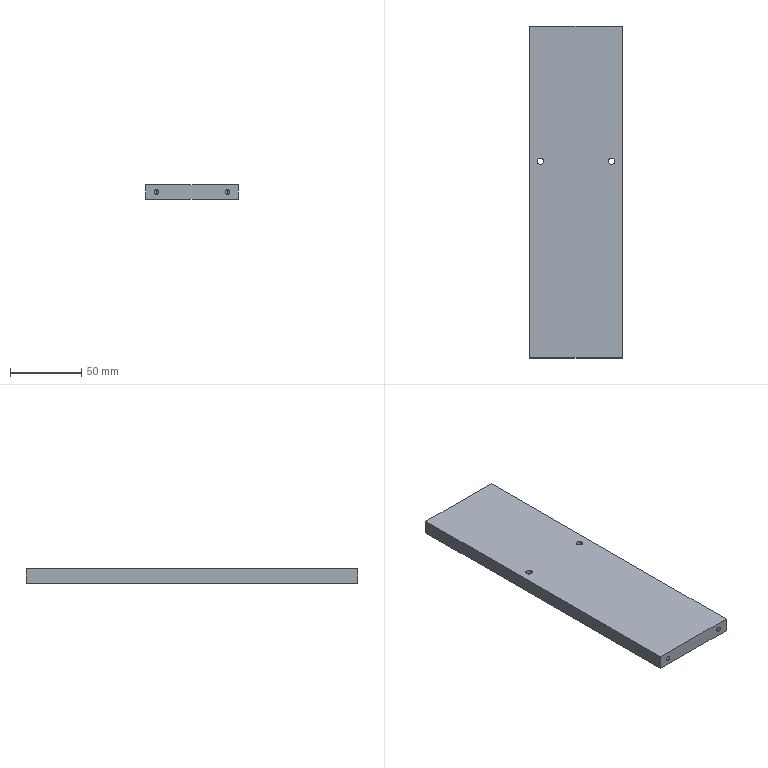Part | SolidWorks | features HoleWzd 2, Extrusion 1, MirrorPattern 1 | 1 solid | 26 faces | box 65 x 233 x 10 mm | volume 150775 mm3 | cylinder 12 | cone 8 | plane 6 | commonest cylinder face diameters 3.3 x8 4.5 x4
STEP:
#1=CARTESIAN_POINT('',(-22.75,21.5,5.));
#2=VERTEX_POINT('',#1);
#3=CARTESIAN_POINT('',(-27.25,21.5,5.));
#4=VERTEX_POINT('',#3);
#5=CARTESIAN_POINT('',(-25.,21.5,5.));
#6=DIRECTION('',(0.,0.,-1.));
#7=DIRECTION('',(-1.,0.,0.));
#8=AXIS2_PLACEMENT_3D('',#5,#6,#7);
#9=CIRCLE('',#8,2.25);
#10=EDGE_CURVE('',#2,#4,#9,.T.);
#11=ORIENTED_EDGE('',*,*,#10,.F.);
#12=CARTESIAN_POINT('',(-22.75,21.5,-5.));
#13=VERTEX_POINT('',#12);
#14=CARTESIAN_POINT('',(-22.75,21.5,-5.));
#15=DIRECTION('',(0.,0.,-1.));
#16=VECTOR('',#15,1000.);
#17=LINE('',#14,#16);
#18=EDGE_CURVE('',#2,#13,#17,.T.);
#19=ORIENTED_EDGE('',*,*,#18,.T.);
#20=CARTESIAN_POINT('',(-27.25,21.5,-5.));
#21=VERTEX_POINT('',#20);
#22=CARTESIAN_POINT('',(-25.,21.5,-5.));
#23=DIRECTION('',(0.,0.,-1.));
#24=DIRECTION('',(-1.,0.,0.));
#25=AXIS2_PLACEMENT_3D('',#22,#23,#24);
#26=CIRCLE('',#25,2.25);
#27=EDGE_CURVE('',#13,#21,#26,.T.);
#28=ORIENTED_EDGE('',*,*,#27,.T.);
#29=CARTESIAN_POINT('',(-27.25,21.5,-5.));
#30=DIRECTION('',(0.,0.,-1.));
#31=VECTOR('',#30,1000.);
#32=LINE('',#29,#31);
#33=EDGE_CURVE('',#4,#21,#32,.T.);
#34=ORIENTED_EDGE('',*,*,#33,.F.);
#35=EDGE_LOOP('',(#11,#19,#28,#34));
#36=FACE_OUTER_BOUND('',#35,.T.);
#37=CARTESIAN_POINT('',(-25.,21.5,-5.));
#38=DIRECTION('',(0.,0.,-1.));
#39=DIRECTION('',(-1.,0.,0.));
#40=AXIS2_PLACEMENT_3D('',#37,#38,#39);
#41=CYLINDRICAL_SURFACE('',#40,2.25);
#42=ADVANCED_FACE('',(#36),#41,.F.);
#43=CARTESIAN_POINT('',(27.25,21.5,5.));
#44=VERTEX_POINT('',#43);
#45=CARTESIAN_POINT('',(22.75,21.5,5.));
#46=VERTEX_POINT('',#45);
#47=CARTESIAN_POINT('',(25.,21.5,5.));
#48=DIRECTION('',(0.,0.,-1.));
#49=DIRECTION('',(-1.,0.,0.));
#50=AXIS2_PLACEMENT_3D('',#47,#48,#49);
#51=CIRCLE('',#50,2.25);
#52=EDGE_CURVE('',#44,#46,#51,.T.);
#53=ORIENTED_EDGE('',*,*,#52,.F.);
#54=CARTESIAN_POINT('',(27.25,21.5,-5.));
#55=VERTEX_POINT('',#54);
#56=CARTESIAN_POINT('',(27.25,21.5,-5.));
#57=DIRECTION('',(0.,0.,-1.));
#58=VECTOR('',#57,1000.);
#59=LINE('',#56,#58);
#60=EDGE_CURVE('',#44,#55,#59,.T.);
#61=ORIENTED_EDGE('',*,*,#60,.T.);
#62=CARTESIAN_POINT('',(22.75,21.5,-5.));
#63=VERTEX_POINT('',#62);
#64=CARTESIAN_POINT('',(25.,21.5,-5.));
#65=DIRECTION('',(0.,0.,-1.));
#66=DIRECTION('',(-1.,0.,0.));
#67=AXIS2_PLACEMENT_3D('',#64,#65,#66);
#68=CIRCLE('',#67,2.25);
#69=EDGE_CURVE('',#55,#63,#68,.T.);
#70=ORIENTED_EDGE('',*,*,#69,.T.);
#71=CARTESIAN_POINT('',(22.75,21.5,-5.));
#72=DIRECTION('',(0.,0.,-1.));
#73=VECTOR('',#72,1000.);
#74=LINE('',#71,#73);
#75=EDGE_CURVE('',#46,#63,#74,.T.);
#76=ORIENTED_EDGE('',*,*,#75,.F.);
#77=EDGE_LOOP('',(#53,#61,#70,#76));
#78=FACE_OUTER_BOUND('',#77,.T.);
#79=CARTESIAN_POINT('',(25.,21.5,-5.));
#80=DIRECTION('',(0.,0.,-1.));
#81=DIRECTION('',(-1.,0.,0.));
#82=AXIS2_PLACEMENT_3D('',#79,#80,#81);
#83=CYLINDRICAL_SURFACE('',#82,2.25);
#84=ADVANCED_FACE('',(#78),#83,.F.);
#85=CARTESIAN_POINT('',(25.,-106.4,1.65));
#86=VERTEX_POINT('',#85);
#87=CARTESIAN_POINT('',(25.,-106.4,-1.65));
#88=VERTEX_POINT('',#87);
#89=CARTESIAN_POINT('',(25.,-106.4,0.));
#90=DIRECTION('',(0.,-1.,0.));
#91=DIRECTION('',(0.,0.,-1.));
#92=AXIS2_PLACEMENT_3D('',#89,#90,#91);
#93=CIRCLE('',#92,1.65);
#94=EDGE_CURVE('',#86,#88,#93,.T.);
#95=ORIENTED_EDGE('',*,*,#94,.F.);
#96=CARTESIAN_POINT('',(25.,-116.5,1.65));
#97=VERTEX_POINT('',#96);
#98=CARTESIAN_POINT('',(25.,-116.5,1.65));
#99=DIRECTION('',(0.,-1.,0.));
#100=VECTOR('',#99,1000.);
#101=LINE('',#98,#100);
#102=EDGE_CURVE('',#86,#97,#101,.T.);
#103=ORIENTED_EDGE('',*,*,#102,.T.);
#104=CARTESIAN_POINT('',(25.,-116.5,-1.65));
#105=VERTEX_POINT('',#104);
#106=CARTESIAN_POINT('',(25.,-116.5,0.));
#107=DIRECTION('',(0.,-1.,0.));
#108=DIRECTION('',(0.,0.,-1.));
#109=AXIS2_PLACEMENT_3D('',#106,#107,#108);
#110=CIRCLE('',#109,1.65);
#111=EDGE_CURVE('',#97,#105,#110,.T.);
#112=ORIENTED_EDGE('',*,*,#111,.T.);
#113=CARTESIAN_POINT('',(25.,-116.5,-1.65));
#114=DIRECTION('',(0.,-1.,0.));
#115=VECTOR('',#114,1000.);
#116=LINE('',#113,#115);
#117=EDGE_CURVE('',#88,#105,#116,.T.);
#118=ORIENTED_EDGE('',*,*,#117,.F.);
#119=EDGE_LOOP('',(#95,#103,#112,#118));
#120=FACE_OUTER_BOUND('',#119,.T.);
#121=CARTESIAN_POINT('',(25.,-116.5,0.));
#122=DIRECTION('',(0.,-1.,0.));
#123=DIRECTION('',(0.,0.,-1.));
#124=AXIS2_PLACEMENT_3D('',#121,#122,#123);
#125=CYLINDRICAL_SURFACE('',#124,1.65);
#126=ADVANCED_FACE('',(#120),#125,.F.);
#127=CARTESIAN_POINT('',(25.,-105.409,0.));
#128=VERTEX_POINT('',#127);
#129=CARTESIAN_POINT('',(25.,-106.4,-1.65));
#130=DIRECTION('',(0.,-0.515,-0.8572));
#131=VECTOR('',#130,1000.);
#132=LINE('',#129,#131);
#133=EDGE_CURVE('',#128,#88,#132,.T.);
#134=ORIENTED_EDGE('',*,*,#133,.F.);
#135=CARTESIAN_POINT('',(25.,-106.4,1.65));
#136=DIRECTION('',(0.,-0.515,0.8572));
#137=VECTOR('',#136,1000.);
#138=LINE('',#135,#137);
#139=EDGE_CURVE('',#128,#86,#138,.T.);
#140=ORIENTED_EDGE('',*,*,#139,.T.);
#141=ORIENTED_EDGE('',*,*,#94,.T.);
#142=EDGE_LOOP('',(#134,#140,#141));
#143=FACE_OUTER_BOUND('',#142,.T.);
#144=CARTESIAN_POINT('',(25.,-106.4,0.));
#145=DIRECTION('',(0.,-1.,0.));
#146=DIRECTION('',(0.,0.,-1.));
#147=AXIS2_PLACEMENT_3D('',#144,#145,#146);
#148=CONICAL_SURFACE('',#147,1.65,1.03);
#149=ADVANCED_FACE('',(#143),#148,.F.);
#150=CARTESIAN_POINT('',(-25.,-106.4,1.65));
#151=VERTEX_POINT('',#150);
#152=CARTESIAN_POINT('',(-25.,-106.4,-1.65));
#153=VERTEX_POINT('',#152);
#154=CARTESIAN_POINT('',(-25.,-106.4,0.));
#155=DIRECTION('',(0.,-1.,0.));
#156=DIRECTION('',(0.,0.,-1.));
#157=AXIS2_PLACEMENT_3D('',#154,#155,#156);
#158=CIRCLE('',#157,1.65);
#159=EDGE_CURVE('',#151,#153,#158,.T.);
#160=ORIENTED_EDGE('',*,*,#159,.F.);
#161=CARTESIAN_POINT('',(-25.,-116.5,1.65));
#162=VERTEX_POINT('',#161);
#163=CARTESIAN_POINT('',(-25.,-116.5,1.65));
#164=DIRECTION('',(0.,-1.,0.));
#165=VECTOR('',#164,1000.);
#166=LINE('',#163,#165);
#167=EDGE_CURVE('',#151,#162,#166,.T.);
#168=ORIENTED_EDGE('',*,*,#167,.T.);
#169=CARTESIAN_POINT('',(-25.,-116.5,-1.65));
#170=VERTEX_POINT('',#169);
#171=CARTESIAN_POINT('',(-25.,-116.5,0.));
#172=DIRECTION('',(0.,-1.,0.));
#173=DIRECTION('',(0.,0.,-1.));
#174=AXIS2_PLACEMENT_3D('',#171,#172,#173);
#175=CIRCLE('',#174,1.65);
#176=EDGE_CURVE('',#162,#170,#175,.T.);
#177=ORIENTED_EDGE('',*,*,#176,.T.);
#178=CARTESIAN_POINT('',(-25.,-116.5,-1.65));
#179=DIRECTION('',(0.,-1.,0.));
#180=VECTOR('',#179,1000.);
#181=LINE('',#178,#180);
#182=EDGE_CURVE('',#153,#170,#181,.T.);
#183=ORIENTED_EDGE('',*,*,#182,.F.);
#184=EDGE_LOOP('',(#160,#168,#177,#183));
#185=FACE_OUTER_BOUND('',#184,.T.);
#186=CARTESIAN_POINT('',(-25.,-116.5,0.));
#187=DIRECTION('',(0.,-1.,0.));
#188=DIRECTION('',(0.,0.,-1.));
#189=AXIS2_PLACEMENT_3D('',#186,#187,#188);
#190=CYLINDRICAL_SURFACE('',#189,1.65);
#191=ADVANCED_FACE('',(#185),#190,.F.);
#192=CARTESIAN_POINT('',(-25.,-105.409,0.));
#193=VERTEX_POINT('',#192);
#194=CARTESIAN_POINT('',(-25.,-106.4,-1.65));
#195=DIRECTION('',(0.,-0.515,-0.8572));
#196=VECTOR('',#195,1000.);
#197=LINE('',#194,#196);
#198=EDGE_CURVE('',#193,#153,#197,.T.);
#199=ORIENTED_EDGE('',*,*,#198,.F.);
#200=CARTESIAN_POINT('',(-25.,-106.4,1.65));
#201=DIRECTION('',(0.,-0.515,0.8572));
#202=VECTOR('',#201,1000.);
#203=LINE('',#200,#202);
#204=EDGE_CURVE('',#193,#151,#203,.T.);
#205=ORIENTED_EDGE('',*,*,#204,.T.);
#206=ORIENTED_EDGE('',*,*,#159,.T.);
#207=EDGE_LOOP('',(#199,#205,#206));
#208=FACE_OUTER_BOUND('',#207,.T.);
#209=CARTESIAN_POINT('',(-25.,-106.4,0.));
#210=DIRECTION('',(0.,-1.,0.));
#211=DIRECTION('',(0.,0.,-1.));
#212=AXIS2_PLACEMENT_3D('',#209,#210,#211);
#213=CONICAL_SURFACE('',#212,1.65,1.03);
#214=ADVANCED_FACE('',(#208),#213,.F.);
#215=CARTESIAN_POINT('',(25.,106.4,-1.65));
#216=VERTEX_POINT('',#215);
#217=CARTESIAN_POINT('',(25.,106.4,1.65));
#218=VERTEX_POINT('',#217);
#219=CARTESIAN_POINT('',(25.,106.4,0.));
#220=DIRECTION('',(0.,1.,0.));
#221=DIRECTION('',(0.,0.,1.));
#222=AXIS2_PLACEMENT_3D('',#219,#220,#221);
#223=CIRCLE('',#222,1.65);
#224=EDGE_CURVE('',#216,#218,#223,.T.);
#225=ORIENTED_EDGE('',*,*,#224,.F.);
#226=CARTESIAN_POINT('',(25.,116.5,-1.65));
#227=VERTEX_POINT('',#226);
#228=CARTESIAN_POINT('',(25.,116.5,-1.65));
#229=DIRECTION('',(0.,1.,0.));
#230=VECTOR('',#229,1000.);
#231=LINE('',#228,#230);
#232=EDGE_CURVE('',#216,#227,#231,.T.);
#233=ORIENTED_EDGE('',*,*,#232,.T.);
#234=CARTESIAN_POINT('',(25.,116.5,1.65));
#235=VERTEX_POINT('',#234);
#236=CARTESIAN_POINT('',(25.,116.5,0.));
#237=DIRECTION('',(0.,1.,0.));
#238=DIRECTION('',(0.,0.,1.));
#239=AXIS2_PLACEMENT_3D('',#236,#237,#238);
#240=CIRCLE('',#239,1.65);
#241=EDGE_CURVE('',#227,#235,#240,.T.);
#242=ORIENTED_EDGE('',*,*,#241,.T.);
#243=CARTESIAN_POINT('',(25.,116.5,1.65));
#244=DIRECTION('',(0.,1.,0.));
#245=VECTOR('',#244,1000.);
#246=LINE('',#243,#245);
#247=EDGE_CURVE('',#218,#235,#246,.T.);
#248=ORIENTED_EDGE('',*,*,#247,.F.);
#249=EDGE_LOOP('',(#225,#233,#242,#248));
#250=FACE_OUTER_BOUND('',#249,.T.);
#251=CARTESIAN_POINT('',(25.,116.5,0.));
#252=DIRECTION('',(0.,1.,0.));
#253=DIRECTION('',(0.,0.,1.));
#254=AXIS2_PLACEMENT_3D('',#251,#252,#253);
#255=CYLINDRICAL_SURFACE('',#254,1.65);
#256=ADVANCED_FACE('',(#250),#255,.F.);
#257=CARTESIAN_POINT('',(25.,105.409,0.));
#258=VERTEX_POINT('',#257);
#259=CARTESIAN_POINT('',(25.,106.4,1.65));
#260=DIRECTION('',(0.,0.515,0.8572));
#261=VECTOR('',#260,1000.);
#262=LINE('',#259,#261);
#263=EDGE_CURVE('',#258,#218,#262,.T.);
#264=ORIENTED_EDGE('',*,*,#263,.F.);
#265=CARTESIAN_POINT('',(25.,106.4,-1.65));
#266=DIRECTION('',(0.,0.515,-0.8572));
#267=VECTOR('',#266,1000.);
#268=LINE('',#265,#267);
#269=EDGE_CURVE('',#258,#216,#268,.T.);
#270=ORIENTED_EDGE('',*,*,#269,.T.);
#271=ORIENTED_EDGE('',*,*,#224,.T.);
#272=EDGE_LOOP('',(#264,#270,#271));
#273=FACE_OUTER_BOUND('',#272,.T.);
#274=CARTESIAN_POINT('',(25.,106.4,0.));
#275=DIRECTION('',(0.,1.,0.));
#276=DIRECTION('',(0.,0.,1.));
#277=AXIS2_PLACEMENT_3D('',#274,#275,#276);
#278=CONICAL_SURFACE('',#277,1.65,1.03);
#279=ADVANCED_FACE('',(#273),#278,.F.);
#280=CARTESIAN_POINT('',(-25.,106.4,-1.65));
#281=VERTEX_POINT('',#280);
#282=CARTESIAN_POINT('',(-25.,106.4,1.65));
#283=VERTEX_POINT('',#282);
#284=CARTESIAN_POINT('',(-25.,106.4,0.));
#285=DIRECTION('',(0.,1.,0.));
#286=DIRECTION('',(0.,0.,1.));
#287=AXIS2_PLACEMENT_3D('',#284,#285,#286);
#288=CIRCLE('',#287,1.65);
#289=EDGE_CURVE('',#281,#283,#288,.T.);
#290=ORIENTED_EDGE('',*,*,#289,.F.);
#291=CARTESIAN_POINT('',(-25.,116.5,-1.65));
#292=VERTEX_POINT('',#291);
#293=CARTESIAN_POINT('',(-25.,116.5,-1.65));
#294=DIRECTION('',(0.,1.,0.));
#295=VECTOR('',#294,1000.);
#296=LINE('',#293,#295);
#297=EDGE_CURVE('',#281,#292,#296,.T.);
#298=ORIENTED_EDGE('',*,*,#297,.T.);
#299=CARTESIAN_POINT('',(-25.,116.5,1.65));
#300=VERTEX_POINT('',#299);
#301=CARTESIAN_POINT('',(-25.,116.5,0.));
#302=DIRECTION('',(0.,1.,0.));
#303=DIRECTION('',(0.,0.,1.));
#304=AXIS2_PLACEMENT_3D('',#301,#302,#303);
#305=CIRCLE('',#304,1.65);
#306=EDGE_CURVE('',#292,#300,#305,.T.);
#307=ORIENTED_EDGE('',*,*,#306,.T.);
#308=CARTESIAN_POINT('',(-25.,116.5,1.65));
#309=DIRECTION('',(0.,1.,0.));
#310=VECTOR('',#309,1000.);
#311=LINE('',#308,#310);
#312=EDGE_CURVE('',#283,#300,#311,.T.);
#313=ORIENTED_EDGE('',*,*,#312,.F.);
#314=EDGE_LOOP('',(#290,#298,#307,#313));
#315=FACE_OUTER_BOUND('',#314,.T.);
#316=CARTESIAN_POINT('',(-25.,116.5,0.));
#317=DIRECTION('',(0.,1.,0.));
#318=DIRECTION('',(0.,0.,1.));
#319=AXIS2_PLACEMENT_3D('',#316,#317,#318);
#320=CYLINDRICAL_SURFACE('',#319,1.65);
#321=ADVANCED_FACE('',(#315),#320,.F.);
#322=CARTESIAN_POINT('',(-25.,105.409,0.));
#323=VERTEX_POINT('',#322);
#324=CARTESIAN_POINT('',(-25.,106.4,1.65));
#325=DIRECTION('',(0.,0.515,0.8572));
#326=VECTOR('',#325,1000.);
#327=LINE('',#324,#326);
#328=EDGE_CURVE('',#323,#283,#327,.T.);
#329=ORIENTED_EDGE('',*,*,#328,.F.);
#330=CARTESIAN_POINT('',(-25.,106.4,-1.65));
#331=DIRECTION('',(0.,0.515,-0.8572));
#332=VECTOR('',#331,1000.);
#333=LINE('',#330,#332);
#334=EDGE_CURVE('',#323,#281,#333,.T.);
#335=ORIENTED_EDGE('',*,*,#334,.T.);
#336=ORIENTED_EDGE('',*,*,#289,.T.);
#337=EDGE_LOOP('',(#329,#335,#336));
#338=FACE_OUTER_BOUND('',#337,.T.);
#339=CARTESIAN_POINT('',(-25.,106.4,0.));
#340=DIRECTION('',(0.,1.,0.));
#341=DIRECTION('',(0.,0.,1.));
#342=AXIS2_PLACEMENT_3D('',#339,#340,#341);
#343=CONICAL_SURFACE('',#342,1.65,1.03);
#344=ADVANCED_FACE('',(#338),#343,.F.);
#345=CARTESIAN_POINT('',(32.5,-116.5,5.));
#346=VERTEX_POINT('',#345);
#347=CARTESIAN_POINT('',(32.5,-116.5,-5.));
#348=VERTEX_POINT('',#347);
#349=CARTESIAN_POINT('',(32.5,-116.5,-5.));
#350=DIRECTION('',(0.,0.,-1.));
#351=VECTOR('',#350,1000.);
#352=LINE('',#349,#351);
#353=EDGE_CURVE('',#346,#348,#352,.T.);
#354=ORIENTED_EDGE('',*,*,#353,.T.);
#355=CARTESIAN_POINT('',(32.5,116.5,-5.));
#356=VERTEX_POINT('',#355);
#357=CARTESIAN_POINT('',(32.5,116.5,-5.));
#358=DIRECTION('',(0.,-1.,0.));
#359=VECTOR('',#358,1000.);
#360=LINE('',#357,#359);
#361=EDGE_CURVE('',#356,#348,#360,.T.);
#362=ORIENTED_EDGE('',*,*,#361,.F.);
#363=CARTESIAN_POINT('',(32.5,116.5,5.));
#364=VERTEX_POINT('',#363);
#365=CARTESIAN_POINT('',(32.5,116.5,-5.));
#366=DIRECTION('',(0.,0.,-1.));
#367=VECTOR('',#366,1000.);
#368=LINE('',#365,#367);
#369=EDGE_CURVE('',#364,#356,#368,.T.);
#370=ORIENTED_EDGE('',*,*,#369,.F.);
#371=CARTESIAN_POINT('',(32.5,116.5,5.));
#372=DIRECTION('',(0.,-1.,0.));
#373=VECTOR('',#372,1000.);
#374=LINE('',#371,#373);
#375=EDGE_CURVE('',#364,#346,#374,.T.);
#376=ORIENTED_EDGE('',*,*,#375,.T.);
#377=EDGE_LOOP('',(#354,#362,#370,#376));
#378=FACE_OUTER_BOUND('',#377,.T.);
#379=CARTESIAN_POINT('',(32.5,116.5,-5.));
#380=DIRECTION('',(-1.,0.,0.));
#381=DIRECTION('',(0.,0.,1.));
#382=AXIS2_PLACEMENT_3D('',#379,#380,#381);
#383=PLANE('',#382);
#384=ADVANCED_FACE('',(#378),#383,.F.);
#385=CARTESIAN_POINT('',(-25.,21.5,-5.));
#386=DIRECTION('',(0.,0.,-1.));
#387=DIRECTION('',(-1.,0.,0.));
#388=AXIS2_PLACEMENT_3D('',#385,#386,#387);
#389=CIRCLE('',#388,2.25);
#390=EDGE_CURVE('',#21,#13,#389,.T.);
#391=ORIENTED_EDGE('',*,*,#390,.F.);
#392=ORIENTED_EDGE('',*,*,#27,.F.);
#393=EDGE_LOOP('',(#391,#392));
#394=FACE_BOUND('',#393,.T.);
#395=CARTESIAN_POINT('',(25.,21.5,-5.));
#396=DIRECTION('',(0.,0.,-1.));
#397=DIRECTION('',(-1.,0.,0.));
#398=AXIS2_PLACEMENT_3D('',#395,#396,#397);
#399=CIRCLE('',#398,2.25);
#400=EDGE_CURVE('',#63,#55,#399,.T.);
#401=ORIENTED_EDGE('',*,*,#400,.F.);
#402=ORIENTED_EDGE('',*,*,#69,.F.);
#403=EDGE_LOOP('',(#401,#402));
#404=FACE_BOUND('',#403,.T.);
#405=CARTESIAN_POINT('',(-32.5,-116.5,-5.));
#406=VERTEX_POINT('',#405);
#407=CARTESIAN_POINT('',(-32.5,-116.5,-5.));
#408=DIRECTION('',(-1.,0.,0.));
#409=VECTOR('',#408,1000.);
#410=LINE('',#407,#409);
#411=EDGE_CURVE('',#348,#406,#410,.T.);
#412=ORIENTED_EDGE('',*,*,#411,.T.);
#413=CARTESIAN_POINT('',(-32.5,116.5,-5.));
#414=VERTEX_POINT('',#413);
#415=CARTESIAN_POINT('',(-32.5,116.5,-5.));
#416=DIRECTION('',(0.,-1.,0.));
#417=VECTOR('',#416,1000.);
#418=LINE('',#415,#417);
#419=EDGE_CURVE('',#414,#406,#418,.T.);
#420=ORIENTED_EDGE('',*,*,#419,.F.);
#421=CARTESIAN_POINT('',(-32.5,116.5,-5.));
#422=DIRECTION('',(-1.,0.,0.));
#423=VECTOR('',#422,1000.);
#424=LINE('',#421,#423);
#425=EDGE_CURVE('',#356,#414,#424,.T.);
#426=ORIENTED_EDGE('',*,*,#425,.F.);
#427=ORIENTED_EDGE('',*,*,#361,.T.);
#428=EDGE_LOOP('',(#412,#420,#426,#427));
#429=FACE_OUTER_BOUND('',#428,.T.);
#430=CARTESIAN_POINT('',(-32.5,116.5,-5.));
#431=DIRECTION('',(0.,0.,1.));
#432=DIRECTION('',(1.,0.,0.));
#433=AXIS2_PLACEMENT_3D('',#430,#431,#432);
#434=PLANE('',#433);
#435=ADVANCED_FACE('',(#394,#404,#429),#434,.F.);
#436=CARTESIAN_POINT('',(-32.5,-116.5,5.));
#437=VERTEX_POINT('',#436);
#438=CARTESIAN_POINT('',(-32.5,-116.5,-5.));
#439=DIRECTION('',(0.,0.,1.));
#440=VECTOR('',#439,1000.);
#441=LINE('',#438,#440);
#442=EDGE_CURVE('',#406,#437,#441,.T.);
#443=ORIENTED_EDGE('',*,*,#442,.T.);
#444=CARTESIAN_POINT('',(-32.5,116.5,5.));
#445=VERTEX_POINT('',#444);
#446=CARTESIAN_POINT('',(-32.5,116.5,5.));
#447=DIRECTION('',(0.,-1.,0.));
#448=VECTOR('',#447,1000.);
#449=LINE('',#446,#448);
#450=EDGE_CURVE('',#445,#437,#449,.T.);
#451=ORIENTED_EDGE('',*,*,#450,.F.);
#452=CARTESIAN_POINT('',(-32.5,116.5,-5.));
#453=DIRECTION('',(0.,0.,1.));
#454=VECTOR('',#453,1000.);
#455=LINE('',#452,#454);
#456=EDGE_CURVE('',#414,#445,#455,.T.);
#457=ORIENTED_EDGE('',*,*,#456,.F.);
#458=ORIENTED_EDGE('',*,*,#419,.T.);
#459=EDGE_LOOP('',(#443,#451,#457,#458));
#460=FACE_OUTER_BOUND('',#459,.T.);
#461=CARTESIAN_POINT('',(-32.5,116.5,-5.));
#462=DIRECTION('',(1.,0.,0.));
#463=DIRECTION('',(0.,0.,-1.));
#464=AXIS2_PLACEMENT_3D('',#461,#462,#463);
#465=PLANE('',#464);
#466=ADVANCED_FACE('',(#460),#465,.F.);
#467=CARTESIAN_POINT('',(-25.,21.5,5.));
#468=DIRECTION('',(0.,0.,-1.));
#469=DIRECTION('',(-1.,0.,0.));
#470=AXIS2_PLACEMENT_3D('',#467,#468,#469);
#471=CIRCLE('',#470,2.25);
#472=EDGE_CURVE('',#4,#2,#471,.T.);
#473=ORIENTED_EDGE('',*,*,#472,.T.);
#474=ORIENTED_EDGE('',*,*,#10,.T.);
#475=EDGE_LOOP('',(#473,#474));
#476=FACE_BOUND('',#475,.T.);
#477=CARTESIAN_POINT('',(25.,21.5,5.));
#478=DIRECTION('',(0.,0.,-1.));
#479=DIRECTION('',(-1.,0.,0.));
#480=AXIS2_PLACEMENT_3D('',#477,#478,#479);
#481=CIRCLE('',#480,2.25);
#482=EDGE_CURVE('',#46,#44,#481,.T.);
#483=ORIENTED_EDGE('',*,*,#482,.T.);
#484=ORIENTED_EDGE('',*,*,#52,.T.);
#485=EDGE_LOOP('',(#483,#484));
#486=FACE_BOUND('',#485,.T.);
#487=CARTESIAN_POINT('',(-32.5,-116.5,5.));
#488=DIRECTION('',(1.,0.,0.));
#489=VECTOR('',#488,1000.);
#490=LINE('',#487,#489);
#491=EDGE_CURVE('',#437,#346,#490,.T.);
#492=ORIENTED_EDGE('',*,*,#491,.T.);
#493=ORIENTED_EDGE('',*,*,#375,.F.);
#494=CARTESIAN_POINT('',(-32.5,116.5,5.));
#495=DIRECTION('',(1.,0.,0.));
#496=VECTOR('',#495,1000.);
#497=LINE('',#494,#496);
#498=EDGE_CURVE('',#445,#364,#497,.T.);
#499=ORIENTED_EDGE('',*,*,#498,.F.);
#500=ORIENTED_EDGE('',*,*,#450,.T.);
#501=EDGE_LOOP('',(#492,#493,#499,#500));
#502=FACE_OUTER_BOUND('',#501,.T.);
#503=CARTESIAN_POINT('',(-32.5,116.5,5.));
#504=DIRECTION('',(0.,0.,-1.));
#505=DIRECTION('',(-1.,0.,0.));
#506=AXIS2_PLACEMENT_3D('',#503,#504,#505);
#507=PLANE('',#506);
#508=ADVANCED_FACE('',(#476,#486,#502),#507,.F.);
#509=CARTESIAN_POINT('',(25.,116.5,0.));
#510=DIRECTION('',(0.,1.,0.));
#511=DIRECTION('',(0.,0.,1.));
#512=AXIS2_PLACEMENT_3D('',#509,#510,#511);
#513=CIRCLE('',#512,1.65);
#514=EDGE_CURVE('',#235,#227,#513,.T.);
#515=ORIENTED_EDGE('',*,*,#514,.F.);
#516=ORIENTED_EDGE('',*,*,#241,.F.);
#517=EDGE_LOOP('',(#515,#516));
#518=FACE_BOUND('',#517,.T.);
#519=CARTESIAN_POINT('',(-25.,116.5,0.));
#520=DIRECTION('',(0.,1.,0.));
#521=DIRECTION('',(0.,0.,1.));
#522=AXIS2_PLACEMENT_3D('',#519,#520,#521);
#523=CIRCLE('',#522,1.65);
#524=EDGE_CURVE('',#300,#292,#523,.T.);
#525=ORIENTED_EDGE('',*,*,#524,.F.);
#526=ORIENTED_EDGE('',*,*,#306,.F.);
#527=EDGE_LOOP('',(#525,#526));
#528=FACE_BOUND('',#527,.T.);
#529=ORIENTED_EDGE('',*,*,#369,.T.);
#530=ORIENTED_EDGE('',*,*,#425,.T.);
#531=ORIENTED_EDGE('',*,*,#456,.T.);
#532=ORIENTED_EDGE('',*,*,#498,.T.);
#533=EDGE_LOOP('',(#529,#530,#531,#532));
#534=FACE_OUTER_BOUND('',#533,.T.);
#535=CARTESIAN_POINT('',(0.,116.5,0.));
#536=DIRECTION('',(0.,1.,0.));
#537=DIRECTION('',(0.,0.,1.));
#538=AXIS2_PLACEMENT_3D('',#535,#536,#537);
#539=PLANE('',#538);
#540=ADVANCED_FACE('',(#518,#528,#534),#539,.T.);
#541=CARTESIAN_POINT('',(25.,-116.5,0.));
#542=DIRECTION('',(0.,-1.,0.));
#543=DIRECTION('',(0.,0.,-1.));
#544=AXIS2_PLACEMENT_3D('',#541,#542,#543);
#545=CIRCLE('',#544,1.65);
#546=EDGE_CURVE('',#105,#97,#545,.T.);
#547=ORIENTED_EDGE('',*,*,#546,.F.);
#548=ORIENTED_EDGE('',*,*,#111,.F.);
#549=EDGE_LOOP('',(#547,#548));
#550=FACE_BOUND('',#549,.T.);
#551=CARTESIAN_POINT('',(-25.,-116.5,0.));
#552=DIRECTION('',(0.,-1.,0.));
#553=DIRECTION('',(0.,0.,-1.));
#554=AXIS2_PLACEMENT_3D('',#551,#552,#553);
#555=CIRCLE('',#554,1.65);
#556=EDGE_CURVE('',#170,#162,#555,.T.);
#557=ORIENTED_EDGE('',*,*,#556,.F.);
#558=ORIENTED_EDGE('',*,*,#176,.F.);
#559=EDGE_LOOP('',(#557,#558));
#560=FACE_BOUND('',#559,.T.);
#561=ORIENTED_EDGE('',*,*,#353,.F.);
#562=ORIENTED_EDGE('',*,*,#491,.F.);
#563=ORIENTED_EDGE('',*,*,#442,.F.);
#564=ORIENTED_EDGE('',*,*,#411,.F.);
#565=EDGE_LOOP('',(#561,#562,#563,#564));
#566=FACE_OUTER_BOUND('',#565,.T.);
#567=CARTESIAN_POINT('',(0.,-116.5,0.));
#568=DIRECTION('',(0.,1.,0.));
#569=DIRECTION('',(0.,0.,1.));
#570=AXIS2_PLACEMENT_3D('',#567,#568,#569);
#571=PLANE('',#570);
#572=ADVANCED_FACE('',(#550,#560,#566),#571,.F.);
#573=ORIENTED_EDGE('',*,*,#334,.F.);
#574=ORIENTED_EDGE('',*,*,#328,.T.);
#575=CARTESIAN_POINT('',(-25.,106.4,0.));
#576=DIRECTION('',(0.,1.,0.));
#577=DIRECTION('',(0.,0.,1.));
#578=AXIS2_PLACEMENT_3D('',#575,#576,#577);
#579=CIRCLE('',#578,1.65);
#580=EDGE_CURVE('',#283,#281,#579,.T.);
#581=ORIENTED_EDGE('',*,*,#580,.T.);
#582=EDGE_LOOP('',(#573,#574,#581));
#583=FACE_OUTER_BOUND('',#582,.T.);
#584=CARTESIAN_POINT('',(-25.,106.4,0.));
#585=DIRECTION('',(0.,1.,0.));
#586=DIRECTION('',(0.,0.,1.));
#587=AXIS2_PLACEMENT_3D('',#584,#585,#586);
#588=CONICAL_SURFACE('',#587,1.65,1.03);
#589=ADVANCED_FACE('',(#583),#588,.F.);
#590=ORIENTED_EDGE('',*,*,#297,.F.);
#591=ORIENTED_EDGE('',*,*,#580,.F.);
#592=ORIENTED_EDGE('',*,*,#312,.T.);
#593=ORIENTED_EDGE('',*,*,#524,.T.);
#594=EDGE_LOOP('',(#590,#591,#592,#593));
#595=FACE_OUTER_BOUND('',#594,.T.);
#596=CARTESIAN_POINT('',(-25.,116.5,0.));
#597=DIRECTION('',(0.,1.,0.));
#598=DIRECTION('',(0.,0.,1.));
#599=AXIS2_PLACEMENT_3D('',#596,#597,#598);
#600=CYLINDRICAL_SURFACE('',#599,1.65);
#601=ADVANCED_FACE('',(#595),#600,.F.);
#602=ORIENTED_EDGE('',*,*,#269,.F.);
#603=ORIENTED_EDGE('',*,*,#263,.T.);
#604=CARTESIAN_POINT('',(25.,106.4,0.));
#605=DIRECTION('',(0.,1.,0.));
#606=DIRECTION('',(0.,0.,1.));
#607=AXIS2_PLACEMENT_3D('',#604,#605,#606);
#608=CIRCLE('',#607,1.65);
#609=EDGE_CURVE('',#218,#216,#608,.T.);
#610=ORIENTED_EDGE('',*,*,#609,.T.);
#611=EDGE_LOOP('',(#602,#603,#610));
#612=FACE_OUTER_BOUND('',#611,.T.);
#613=CARTESIAN_POINT('',(25.,106.4,0.));
#614=DIRECTION('',(0.,1.,0.));
#615=DIRECTION('',(0.,0.,1.));
#616=AXIS2_PLACEMENT_3D('',#613,#614,#615);
#617=CONICAL_SURFACE('',#616,1.65,1.03);
#618=ADVANCED_FACE('',(#612),#617,.F.);
#619=ORIENTED_EDGE('',*,*,#232,.F.);
#620=ORIENTED_EDGE('',*,*,#609,.F.);
#621=ORIENTED_EDGE('',*,*,#247,.T.);
#622=ORIENTED_EDGE('',*,*,#514,.T.);
#623=EDGE_LOOP('',(#619,#620,#621,#622));
#624=FACE_OUTER_BOUND('',#623,.T.);
#625=CARTESIAN_POINT('',(25.,116.5,0.));
#626=DIRECTION('',(0.,1.,0.));
#627=DIRECTION('',(0.,0.,1.));
#628=AXIS2_PLACEMENT_3D('',#625,#626,#627);
#629=CYLINDRICAL_SURFACE('',#628,1.65);
#630=ADVANCED_FACE('',(#624),#629,.F.);
#631=ORIENTED_EDGE('',*,*,#204,.F.);
#632=ORIENTED_EDGE('',*,*,#198,.T.);
#633=CARTESIAN_POINT('',(-25.,-106.4,0.));
#634=DIRECTION('',(0.,-1.,0.));
#635=DIRECTION('',(0.,0.,-1.));
#636=AXIS2_PLACEMENT_3D('',#633,#634,#635);
#637=CIRCLE('',#636,1.65);
#638=EDGE_CURVE('',#153,#151,#637,.T.);
#639=ORIENTED_EDGE('',*,*,#638,.T.);
#640=EDGE_LOOP('',(#631,#632,#639));
#641=FACE_OUTER_BOUND('',#640,.T.);
#642=CARTESIAN_POINT('',(-25.,-106.4,0.));
#643=DIRECTION('',(0.,-1.,0.));
#644=DIRECTION('',(0.,0.,-1.));
#645=AXIS2_PLACEMENT_3D('',#642,#643,#644);
#646=CONICAL_SURFACE('',#645,1.65,1.03);
#647=ADVANCED_FACE('',(#641),#646,.F.);
#648=ORIENTED_EDGE('',*,*,#167,.F.);
#649=ORIENTED_EDGE('',*,*,#638,.F.);
#650=ORIENTED_EDGE('',*,*,#182,.T.);
#651=ORIENTED_EDGE('',*,*,#556,.T.);
#652=EDGE_LOOP('',(#648,#649,#650,#651));
#653=FACE_OUTER_BOUND('',#652,.T.);
#654=CARTESIAN_POINT('',(-25.,-116.5,0.));
#655=DIRECTION('',(0.,-1.,0.));
#656=DIRECTION('',(0.,0.,-1.));
#657=AXIS2_PLACEMENT_3D('',#654,#655,#656);
#658=CYLINDRICAL_SURFACE('',#657,1.65);
#659=ADVANCED_FACE('',(#653),#658,.F.);
#660=ORIENTED_EDGE('',*,*,#139,.F.);
#661=ORIENTED_EDGE('',*,*,#133,.T.);
#662=CARTESIAN_POINT('',(25.,-106.4,0.));
#663=DIRECTION('',(0.,-1.,0.));
#664=DIRECTION('',(0.,0.,-1.));
#665=AXIS2_PLACEMENT_3D('',#662,#663,#664);
#666=CIRCLE('',#665,1.65);
#667=EDGE_CURVE('',#88,#86,#666,.T.);
#668=ORIENTED_EDGE('',*,*,#667,.T.);
#669=EDGE_LOOP('',(#660,#661,#668));
#670=FACE_OUTER_BOUND('',#669,.T.);
#671=CARTESIAN_POINT('',(25.,-106.4,0.));
#672=DIRECTION('',(0.,-1.,0.));
#673=DIRECTION('',(0.,0.,-1.));
#674=AXIS2_PLACEMENT_3D('',#671,#672,#673);
#675=CONICAL_SURFACE('',#674,1.65,1.03);
#676=ADVANCED_FACE('',(#670),#675,.F.);
#677=ORIENTED_EDGE('',*,*,#102,.F.);
#678=ORIENTED_EDGE('',*,*,#667,.F.);
#679=ORIENTED_EDGE('',*,*,#117,.T.);
#680=ORIENTED_EDGE('',*,*,#546,.T.);
#681=EDGE_LOOP('',(#677,#678,#679,#680));
#682=FACE_OUTER_BOUND('',#681,.T.);
#683=CARTESIAN_POINT('',(25.,-116.5,0.));
#684=DIRECTION('',(0.,-1.,0.));
#685=DIRECTION('',(0.,0.,-1.));
#686=AXIS2_PLACEMENT_3D('',#683,#684,#685);
#687=CYLINDRICAL_SURFACE('',#686,1.65);
#688=ADVANCED_FACE('',(#682),#687,.F.);
#689=ORIENTED_EDGE('',*,*,#60,.F.);
#690=ORIENTED_EDGE('',*,*,#482,.F.);
#691=ORIENTED_EDGE('',*,*,#75,.T.);
#692=ORIENTED_EDGE('',*,*,#400,.T.);
#693=EDGE_LOOP('',(#689,#690,#691,#692));
#694=FACE_OUTER_BOUND('',#693,.T.);
#695=CARTESIAN_POINT('',(25.,21.5,-5.));
#696=DIRECTION('',(0.,0.,-1.));
#697=DIRECTION('',(-1.,0.,0.));
#698=AXIS2_PLACEMENT_3D('',#695,#696,#697);
#699=CYLINDRICAL_SURFACE('',#698,2.25);
#700=ADVANCED_FACE('',(#694),#699,.F.);
#701=ORIENTED_EDGE('',*,*,#18,.F.);
#702=ORIENTED_EDGE('',*,*,#472,.F.);
#703=ORIENTED_EDGE('',*,*,#33,.T.);
#704=ORIENTED_EDGE('',*,*,#390,.T.);
#705=EDGE_LOOP('',(#701,#702,#703,#704));
#706=FACE_OUTER_BOUND('',#705,.T.);
#707=CARTESIAN_POINT('',(-25.,21.5,-5.));
#708=DIRECTION('',(0.,0.,-1.));
#709=DIRECTION('',(-1.,0.,0.));
#710=AXIS2_PLACEMENT_3D('',#707,#708,#709);
#711=CYLINDRICAL_SURFACE('',#710,2.25);
#712=ADVANCED_FACE('',(#706),#711,.F.);
#713=CLOSED_SHELL('',(#42,#84,#126,#149,#191,#214,#256,#279,#321,#344,#384,#435,#466,#508,#540,#572,#589,#601,#618,#630,#647,#659,#676,#688,#700,#712));
#714=MANIFOLD_SOLID_BREP('',#713);
#715=CARTESIAN_POINT('',(0.,0.,0.));
#716=DIRECTION('',(0.,0.,1.));
#717=DIRECTION('',(1.,0.,0.));
#718=AXIS2_PLACEMENT_3D('',#715,#716,#717);
#719=(LENGTH_UNIT()NAMED_UNIT(*)SI_UNIT(.MILLI.,.METRE.));
#720=UNCERTAINTY_MEASURE_WITH_UNIT(LENGTH_MEASURE(0.00001),#719,'','');
#721=(NAMED_UNIT(*)PLANE_ANGLE_UNIT()SI_UNIT($,.RADIAN.));
#722=(NAMED_UNIT(*)SI_UNIT($,.STERADIAN.)SOLID_ANGLE_UNIT());
#723=(GEOMETRIC_REPRESENTATION_CONTEXT(3)GLOBAL_UNCERTAINTY_ASSIGNED_CONTEXT((#720))GLOBAL_UNIT_ASSIGNED_CONTEXT((#719,#721,#722))REPRESENTATION_CONTEXT('',''));
#724=ADVANCED_BREP_SHAPE_REPRESENTATION('',(#714,#718),#723);